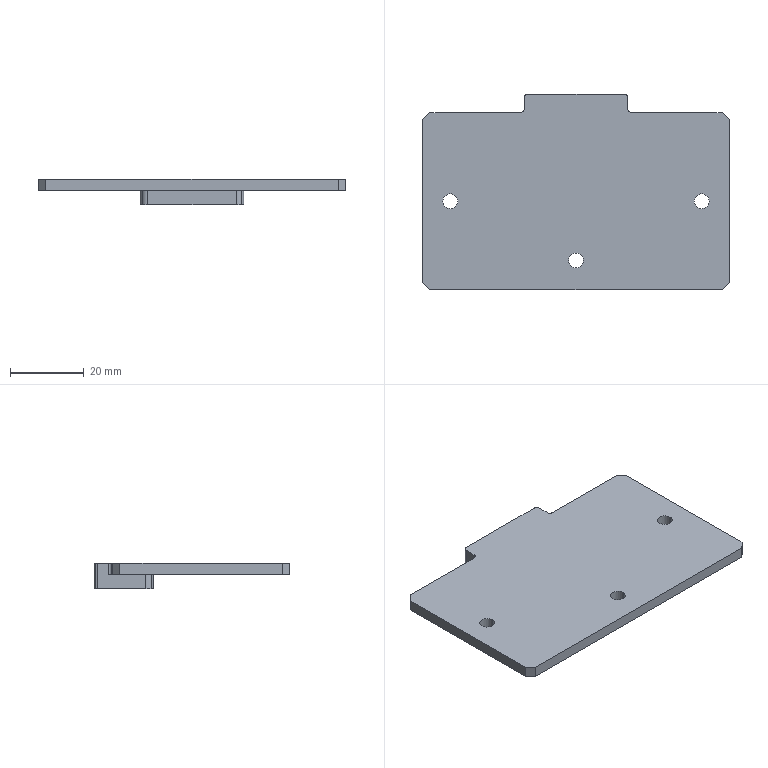Part | STEP file | ASND-0110-Body 1-4 | 1 solid | 41 faces | box 83 x 53 x 7 mm | volume 13678 mm3 | cylinder 21 | plane 20 | commonest cylinder face diameters 2 x11 4 x10